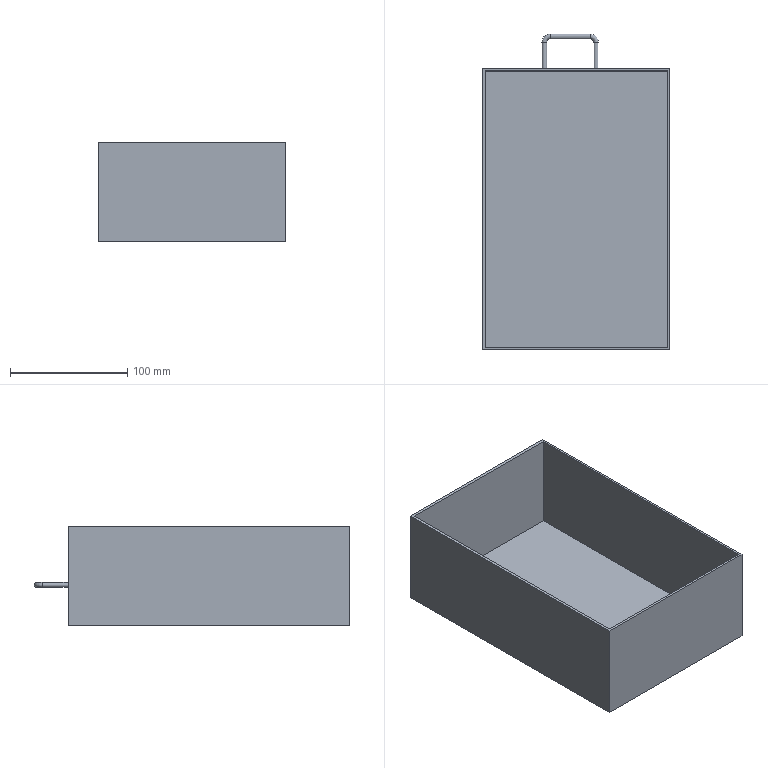Part | NX | features solid 2 | 1 solid | 16 faces | box 160 x 269 x 85 mm | volume 244007 mm3 | plane 11 | cylinder 3 | torus 2 | commonest cylinder face diameters 4 x3
STEP:
#1=CARTESIAN_POINT('',(553.,305.,-243.));
#2=VERTEX_POINT('',#1);
#3=CARTESIAN_POINT('',(553.,305.,-245.));
#4=DIRECTION('',(0.,1.,0.));
#5=DIRECTION('',(0.,0.,1.));
#6=AXIS2_PLACEMENT_3D('',#3,#4,#5);
#7=CIRCLE('',#6,2.);
#8=EDGE_CURVE('',#2,#2,#7,.F.);
#9=ORIENTED_EDGE('',*,*,#8,.T.);
#10=EDGE_LOOP('',(#9));
#11=FACE_BOUND('',#10,.T.);
#12=CARTESIAN_POINT('',(500.,305.,-195.));
#13=VERTEX_POINT('',#12);
#14=CARTESIAN_POINT('',(660.,305.,-195.));
#15=VERTEX_POINT('',#14);
#16=CARTESIAN_POINT('',(210.,305.,-195.));
#17=DIRECTION('',(1.,0.,0.));
#18=VECTOR('',#17,1000.);
#19=LINE('',#16,#18);
#20=EDGE_CURVE('',#13,#15,#19,.T.);
#21=ORIENTED_EDGE('',*,*,#20,.T.);
#22=CARTESIAN_POINT('',(660.,305.,-280.));
#23=VERTEX_POINT('',#22);
#24=CARTESIAN_POINT('',(660.,305.,-160.));
#25=DIRECTION('',(0.,0.,1.));
#26=VECTOR('',#25,1000.);
#27=LINE('',#24,#26);
#28=EDGE_CURVE('',#15,#23,#27,.F.);
#29=ORIENTED_EDGE('',*,*,#28,.T.);
#30=CARTESIAN_POINT('',(500.,305.,-280.));
#31=VERTEX_POINT('',#30);
#32=CARTESIAN_POINT('',(702.5,305.,-280.));
#33=DIRECTION('',(1.,0.,0.));
#34=VECTOR('',#33,1000.);
#35=LINE('',#32,#34);
#36=EDGE_CURVE('',#31,#23,#35,.T.);
#37=ORIENTED_EDGE('',*,*,#36,.F.);
#38=CARTESIAN_POINT('',(500.,305.,-160.));
#39=DIRECTION('',(0.,0.,-1.));
#40=VECTOR('',#39,1000.);
#41=LINE('',#38,#40);
#42=EDGE_CURVE('',#13,#31,#41,.T.);
#43=ORIENTED_EDGE('',*,*,#42,.F.);
#44=EDGE_LOOP('',(#21,#29,#37,#43));
#45=FACE_BOUND('',#44,.T.);
#46=CARTESIAN_POINT('',(597.,305.,-247.));
#47=VERTEX_POINT('',#46);
#48=CARTESIAN_POINT('',(597.,305.,-245.));
#49=DIRECTION('',(0.,-1.,0.));
#50=DIRECTION('',(0.,0.,-1.));
#51=AXIS2_PLACEMENT_3D('',#48,#49,#50);
#52=CIRCLE('',#51,2.);
#53=EDGE_CURVE('',#47,#47,#52,.F.);
#54=ORIENTED_EDGE('',*,*,#53,.F.);
#55=EDGE_LOOP('',(#54));
#56=FACE_BOUND('',#55,.T.);
#57=CARTESIAN_POINT('',(485.,305.,-160.));
#58=DIRECTION('',(0.,-1.,0.));
#59=DIRECTION('',(0.,0.,1.));
#60=AXIS2_PLACEMENT_3D('',#57,#58,#59);
#61=PLANE('',#60);
#62=ADVANCED_FACE('',(#11,#45,#56),#61,.F.);
#63=CARTESIAN_POINT('',(660.,65.,-195.));
#64=VERTEX_POINT('',#63);
#65=CARTESIAN_POINT('',(660.,0.,-195.));
#66=DIRECTION('',(0.,1.,0.));
#67=VECTOR('',#66,1000.);
#68=LINE('',#65,#67);
#69=EDGE_CURVE('',#15,#64,#68,.F.);
#70=ORIENTED_EDGE('',*,*,#69,.T.);
#71=CARTESIAN_POINT('',(660.,65.,-280.));
#72=VERTEX_POINT('',#71);
#73=CARTESIAN_POINT('',(660.,65.,-140.));
#74=DIRECTION('',(0.,0.,-1.));
#75=VECTOR('',#74,1000.);
#76=LINE('',#73,#75);
#77=EDGE_CURVE('',#64,#72,#76,.T.);
#78=ORIENTED_EDGE('',*,*,#77,.T.);
#79=CARTESIAN_POINT('',(660.,0.,-280.));
#80=DIRECTION('',(0.,1.,0.));
#81=VECTOR('',#80,1000.);
#82=LINE('',#79,#81);
#83=EDGE_CURVE('',#23,#72,#82,.F.);
#84=ORIENTED_EDGE('',*,*,#83,.F.);
#85=ORIENTED_EDGE('',*,*,#28,.F.);
#86=EDGE_LOOP('',(#70,#78,#84,#85));
#87=FACE_BOUND('',#86,.T.);
#88=CARTESIAN_POINT('',(660.,0.,-57.002));
#89=DIRECTION('',(-1.,0.,0.));
#90=DIRECTION('',(0.,0.,1.));
#91=AXIS2_PLACEMENT_3D('',#88,#89,#90);
#92=PLANE('',#91);
#93=ADVANCED_FACE('',(#87),#92,.F.);
#94=CARTESIAN_POINT('',(500.,65.,-195.));
#95=VERTEX_POINT('',#94);
#96=CARTESIAN_POINT('',(500.,0.,-195.));
#97=DIRECTION('',(0.,1.,0.));
#98=VECTOR('',#97,1000.);
#99=LINE('',#96,#98);
#100=EDGE_CURVE('',#95,#13,#99,.T.);
#101=ORIENTED_EDGE('',*,*,#100,.T.);
#102=ORIENTED_EDGE('',*,*,#42,.T.);
#103=CARTESIAN_POINT('',(500.,65.,-280.));
#104=VERTEX_POINT('',#103);
#105=CARTESIAN_POINT('',(500.,-47.5,-280.));
#106=DIRECTION('',(0.,1.,0.));
#107=VECTOR('',#106,1000.);
#108=LINE('',#105,#107);
#109=EDGE_CURVE('',#104,#31,#108,.T.);
#110=ORIENTED_EDGE('',*,*,#109,.F.);
#111=CARTESIAN_POINT('',(500.,65.,-160.));
#112=DIRECTION('',(0.,0.,1.));
#113=VECTOR('',#112,1000.);
#114=LINE('',#111,#113);
#115=EDGE_CURVE('',#95,#104,#114,.F.);
#116=ORIENTED_EDGE('',*,*,#115,.F.);
#117=EDGE_LOOP('',(#101,#102,#110,#116));
#118=FACE_BOUND('',#117,.T.);
#119=CARTESIAN_POINT('',(500.,302.5,-160.));
#120=DIRECTION('',(1.,0.,0.));
#121=DIRECTION('',(0.,0.,-1.));
#122=AXIS2_PLACEMENT_3D('',#119,#120,#121);
#123=PLANE('',#122);
#124=ADVANCED_FACE('',(#118),#123,.F.);
#125=CARTESIAN_POINT('',(-430.,65.,-195.));
#126=DIRECTION('',(1.,0.,0.));
#127=VECTOR('',#126,1000.);
#128=LINE('',#125,#127);
#129=EDGE_CURVE('',#64,#95,#128,.F.);
#130=ORIENTED_EDGE('',*,*,#129,.T.);
#131=ORIENTED_EDGE('',*,*,#115,.T.);
#132=CARTESIAN_POINT('',(-430.,65.,-280.));
#133=DIRECTION('',(1.,0.,0.));
#134=VECTOR('',#133,1000.);
#135=LINE('',#132,#134);
#136=EDGE_CURVE('',#72,#104,#135,.F.);
#137=ORIENTED_EDGE('',*,*,#136,.F.);
#138=ORIENTED_EDGE('',*,*,#77,.F.);
#139=EDGE_LOOP('',(#130,#131,#137,#138));
#140=FACE_BOUND('',#139,.T.);
#141=CARTESIAN_POINT('',(-430.,65.,-140.));
#142=DIRECTION('',(0.,1.,0.));
#143=DIRECTION('',(1.,0.,0.));
#144=AXIS2_PLACEMENT_3D('',#141,#142,#143);
#145=PLANE('',#144);
#146=ADVANCED_FACE('',(#140),#145,.F.);
#147=ORIENTED_EDGE('',*,*,#136,.T.);
#148=ORIENTED_EDGE('',*,*,#109,.T.);
#149=ORIENTED_EDGE('',*,*,#36,.T.);
#150=ORIENTED_EDGE('',*,*,#83,.T.);
#151=EDGE_LOOP('',(#147,#148,#149,#150));
#152=FACE_BOUND('',#151,.T.);
#153=CARTESIAN_POINT('',(702.5,-47.5,-280.));
#154=DIRECTION('',(0.,0.,1.));
#155=DIRECTION('',(1.,0.,0.));
#156=AXIS2_PLACEMENT_3D('',#153,#154,#155);
#157=PLANE('',#156);
#158=ADVANCED_FACE('',(#152),#157,.F.);
#159=CARTESIAN_POINT('',(658.,302.5,-195.));
#160=VERTEX_POINT('',#159);
#161=CARTESIAN_POINT('',(502.5,302.5,-195.));
#162=VERTEX_POINT('',#161);
#163=CARTESIAN_POINT('',(210.,302.5,-195.));
#164=DIRECTION('',(-1.,0.,0.));
#165=VECTOR('',#164,1000.);
#166=LINE('',#163,#165);
#167=EDGE_CURVE('',#160,#162,#166,.T.);
#168=ORIENTED_EDGE('',*,*,#167,.F.);
#169=CARTESIAN_POINT('',(658.,67.,-195.));
#170=VERTEX_POINT('',#169);
#171=CARTESIAN_POINT('',(658.,0.,-195.));
#172=DIRECTION('',(0.,1.,0.));
#173=VECTOR('',#172,1000.);
#174=LINE('',#171,#173);
#175=EDGE_CURVE('',#170,#160,#174,.T.);
#176=ORIENTED_EDGE('',*,*,#175,.F.);
#177=CARTESIAN_POINT('',(502.5,67.,-195.));
#178=VERTEX_POINT('',#177);
#179=CARTESIAN_POINT('',(210.,67.,-195.));
#180=DIRECTION('',(1.,0.,0.));
#181=VECTOR('',#180,1000.);
#182=LINE('',#179,#181);
#183=EDGE_CURVE('',#178,#170,#182,.T.);
#184=ORIENTED_EDGE('',*,*,#183,.F.);
#185=CARTESIAN_POINT('',(502.5,0.,-195.));
#186=DIRECTION('',(0.,-1.,0.));
#187=VECTOR('',#186,1000.);
#188=LINE('',#185,#187);
#189=EDGE_CURVE('',#162,#178,#188,.T.);
#190=ORIENTED_EDGE('',*,*,#189,.F.);
#191=EDGE_LOOP('',(#168,#176,#184,#190));
#192=FACE_BOUND('',#191,.T.);
#193=ORIENTED_EDGE('',*,*,#100,.F.);
#194=ORIENTED_EDGE('',*,*,#129,.F.);
#195=ORIENTED_EDGE('',*,*,#69,.F.);
#196=ORIENTED_EDGE('',*,*,#20,.F.);
#197=EDGE_LOOP('',(#193,#194,#195,#196));
#198=FACE_BOUND('',#197,.T.);
#199=CARTESIAN_POINT('',(210.,0.,-195.));
#200=DIRECTION('',(0.,0.,1.));
#201=DIRECTION('',(1.,0.,0.));
#202=AXIS2_PLACEMENT_3D('',#199,#200,#201);
#203=PLANE('',#202);
#204=ADVANCED_FACE('',(#192,#198),#203,.T.);
#205=CARTESIAN_POINT('',(658.,302.5,-277.5));
#206=VERTEX_POINT('',#205);
#207=CARTESIAN_POINT('',(658.,67.,-277.5));
#208=VERTEX_POINT('',#207);
#209=CARTESIAN_POINT('',(658.,-47.5,-277.5));
#210=DIRECTION('',(0.,-1.,0.));
#211=VECTOR('',#210,1000.);
#212=LINE('',#209,#211);
#213=EDGE_CURVE('',#206,#208,#212,.T.);
#214=ORIENTED_EDGE('',*,*,#213,.F.);
#215=CARTESIAN_POINT('',(502.5,302.5,-277.5));
#216=VERTEX_POINT('',#215);
#217=CARTESIAN_POINT('',(705.,302.5,-277.5));
#218=DIRECTION('',(1.,0.,0.));
#219=VECTOR('',#218,1000.);
#220=LINE('',#217,#219);
#221=EDGE_CURVE('',#216,#206,#220,.T.);
#222=ORIENTED_EDGE('',*,*,#221,.F.);
#223=CARTESIAN_POINT('',(502.5,67.,-277.5));
#224=VERTEX_POINT('',#223);
#225=CARTESIAN_POINT('',(502.5,302.5,-277.5));
#226=DIRECTION('',(0.,1.,0.));
#227=VECTOR('',#226,1000.);
#228=LINE('',#225,#227);
#229=EDGE_CURVE('',#224,#216,#228,.T.);
#230=ORIENTED_EDGE('',*,*,#229,.F.);
#231=CARTESIAN_POINT('',(485.,67.,-277.5));
#232=DIRECTION('',(-1.,0.,0.));
#233=VECTOR('',#232,1000.);
#234=LINE('',#231,#233);
#235=EDGE_CURVE('',#208,#224,#234,.T.);
#236=ORIENTED_EDGE('',*,*,#235,.F.);
#237=EDGE_LOOP('',(#214,#222,#230,#236));
#238=FACE_BOUND('',#237,.T.);
#239=CARTESIAN_POINT('',(702.5,-47.5,-277.5));
#240=DIRECTION('',(0.,0.,1.));
#241=DIRECTION('',(1.,0.,0.));
#242=AXIS2_PLACEMENT_3D('',#239,#240,#241);
#243=PLANE('',#242);
#244=ADVANCED_FACE('',(#238),#243,.T.);
#245=ORIENTED_EDGE('',*,*,#175,.T.);
#246=CARTESIAN_POINT('',(658.,302.5,-160.));
#247=DIRECTION('',(0.,0.,-1.));
#248=VECTOR('',#247,1000.);
#249=LINE('',#246,#248);
#250=EDGE_CURVE('',#160,#206,#249,.T.);
#251=ORIENTED_EDGE('',*,*,#250,.T.);
#252=ORIENTED_EDGE('',*,*,#213,.T.);
#253=CARTESIAN_POINT('',(658.,67.,-160.));
#254=DIRECTION('',(0.,0.,-1.));
#255=VECTOR('',#254,1000.);
#256=LINE('',#253,#255);
#257=EDGE_CURVE('',#170,#208,#256,.T.);
#258=ORIENTED_EDGE('',*,*,#257,.F.);
#259=EDGE_LOOP('',(#245,#251,#252,#258));
#260=FACE_BOUND('',#259,.T.);
#261=CARTESIAN_POINT('',(658.,-47.5,-160.));
#262=DIRECTION('',(1.,0.,0.));
#263=DIRECTION('',(0.,0.,-1.));
#264=AXIS2_PLACEMENT_3D('',#261,#262,#263);
#265=PLANE('',#264);
#266=ADVANCED_FACE('',(#260),#265,.F.);
#267=ORIENTED_EDGE('',*,*,#189,.T.);
#268=CARTESIAN_POINT('',(502.5,67.,-160.));
#269=DIRECTION('',(0.,0.,-1.));
#270=VECTOR('',#269,1000.);
#271=LINE('',#268,#270);
#272=EDGE_CURVE('',#178,#224,#271,.T.);
#273=ORIENTED_EDGE('',*,*,#272,.T.);
#274=ORIENTED_EDGE('',*,*,#229,.T.);
#275=CARTESIAN_POINT('',(502.5,302.5,-160.));
#276=DIRECTION('',(0.,0.,-1.));
#277=VECTOR('',#276,1000.);
#278=LINE('',#275,#277);
#279=EDGE_CURVE('',#162,#216,#278,.T.);
#280=ORIENTED_EDGE('',*,*,#279,.F.);
#281=EDGE_LOOP('',(#267,#273,#274,#280));
#282=FACE_BOUND('',#281,.T.);
#283=CARTESIAN_POINT('',(502.5,302.5,-160.));
#284=DIRECTION('',(-1.,0.,0.));
#285=DIRECTION('',(0.,0.,1.));
#286=AXIS2_PLACEMENT_3D('',#283,#284,#285);
#287=PLANE('',#286);
#288=ADVANCED_FACE('',(#282),#287,.F.);
#289=ORIENTED_EDGE('',*,*,#183,.T.);
#290=ORIENTED_EDGE('',*,*,#257,.T.);
#291=ORIENTED_EDGE('',*,*,#235,.T.);
#292=ORIENTED_EDGE('',*,*,#272,.F.);
#293=EDGE_LOOP('',(#289,#290,#291,#292));
#294=FACE_BOUND('',#293,.T.);
#295=CARTESIAN_POINT('',(485.,67.,-160.));
#296=DIRECTION('',(0.,-1.,0.));
#297=DIRECTION('',(0.,0.,1.));
#298=AXIS2_PLACEMENT_3D('',#295,#296,#297);
#299=PLANE('',#298);
#300=ADVANCED_FACE('',(#294),#299,.F.);
#301=ORIENTED_EDGE('',*,*,#167,.T.);
#302=ORIENTED_EDGE('',*,*,#279,.T.);
#303=ORIENTED_EDGE('',*,*,#221,.T.);
#304=ORIENTED_EDGE('',*,*,#250,.F.);
#305=EDGE_LOOP('',(#301,#302,#303,#304));
#306=FACE_BOUND('',#305,.T.);
#307=CARTESIAN_POINT('',(705.,302.5,-160.));
#308=DIRECTION('',(0.,1.,0.));
#309=DIRECTION('',(0.,0.,-1.));
#310=AXIS2_PLACEMENT_3D('',#307,#308,#309);
#311=PLANE('',#310);
#312=ADVANCED_FACE('',(#306),#311,.F.);
#313=CARTESIAN_POINT('',(558.,332.,-247.));
#314=VERTEX_POINT('',#313);
#315=CARTESIAN_POINT('',(558.,332.,-245.));
#316=DIRECTION('',(1.,0.,0.));
#317=DIRECTION('',(0.,0.,-1.));
#318=AXIS2_PLACEMENT_3D('',#315,#316,#317);
#319=CIRCLE('',#318,2.);
#320=EDGE_CURVE('',#314,#314,#319,.T.);
#321=ORIENTED_EDGE('',*,*,#320,.F.);
#322=EDGE_LOOP('',(#321));
#323=FACE_BOUND('',#322,.T.);
#324=CARTESIAN_POINT('',(553.,327.,-247.));
#325=VERTEX_POINT('',#324);
#326=CARTESIAN_POINT('',(553.,327.,-245.));
#327=DIRECTION('',(0.,1.,0.));
#328=DIRECTION('',(0.,0.,-1.));
#329=AXIS2_PLACEMENT_3D('',#326,#327,#328);
#330=CIRCLE('',#329,2.);
#331=EDGE_CURVE('',#325,#325,#330,.T.);
#332=ORIENTED_EDGE('',*,*,#331,.T.);
#333=EDGE_LOOP('',(#332));
#334=FACE_BOUND('',#333,.T.);
#335=CARTESIAN_POINT('',(558.,327.,-245.));
#336=DIRECTION('',(0.,0.,-1.));
#337=DIRECTION('',(-1.,0.,0.));
#338=AXIS2_PLACEMENT_3D('',#335,#336,#337);
#339=TOROIDAL_SURFACE('',#338,5.,2.);
#340=ADVANCED_FACE('',(#323,#334),#339,.T.);
#341=ORIENTED_EDGE('',*,*,#331,.F.);
#342=EDGE_LOOP('',(#341));
#343=FACE_BOUND('',#342,.T.);
#344=ORIENTED_EDGE('',*,*,#8,.F.);
#345=EDGE_LOOP('',(#344));
#346=FACE_BOUND('',#345,.T.);
#347=CARTESIAN_POINT('',(553.,327.,-245.));
#348=DIRECTION('',(0.,-1.,0.));
#349=DIRECTION('',(0.,0.,1.));
#350=AXIS2_PLACEMENT_3D('',#347,#348,#349);
#351=CYLINDRICAL_SURFACE('',#350,2.);
#352=ADVANCED_FACE('',(#343,#346),#351,.T.);
#353=CARTESIAN_POINT('',(592.,332.,-247.));
#354=VERTEX_POINT('',#353);
#355=CARTESIAN_POINT('',(592.,332.,-245.));
#356=DIRECTION('',(1.,0.,0.));
#357=DIRECTION('',(0.,0.,-1.));
#358=AXIS2_PLACEMENT_3D('',#355,#356,#357);
#359=CIRCLE('',#358,2.);
#360=EDGE_CURVE('',#354,#354,#359,.T.);
#361=ORIENTED_EDGE('',*,*,#360,.F.);
#362=EDGE_LOOP('',(#361));
#363=FACE_BOUND('',#362,.T.);
#364=ORIENTED_EDGE('',*,*,#320,.T.);
#365=EDGE_LOOP('',(#364));
#366=FACE_BOUND('',#365,.T.);
#367=CARTESIAN_POINT('',(592.,332.,-245.));
#368=DIRECTION('',(-1.,0.,0.));
#369=DIRECTION('',(0.,0.,1.));
#370=AXIS2_PLACEMENT_3D('',#367,#368,#369);
#371=CYLINDRICAL_SURFACE('',#370,2.);
#372=ADVANCED_FACE('',(#363,#366),#371,.T.);
#373=CARTESIAN_POINT('',(597.,327.,-247.));
#374=VERTEX_POINT('',#373);
#375=CARTESIAN_POINT('',(597.,327.,-245.));
#376=DIRECTION('',(0.,-1.,0.));
#377=DIRECTION('',(0.,0.,-1.));
#378=AXIS2_PLACEMENT_3D('',#375,#376,#377);
#379=CIRCLE('',#378,2.);
#380=EDGE_CURVE('',#374,#374,#379,.T.);
#381=ORIENTED_EDGE('',*,*,#380,.F.);
#382=EDGE_LOOP('',(#381));
#383=FACE_BOUND('',#382,.T.);
#384=ORIENTED_EDGE('',*,*,#360,.T.);
#385=EDGE_LOOP('',(#384));
#386=FACE_BOUND('',#385,.T.);
#387=CARTESIAN_POINT('',(592.,327.,-245.));
#388=DIRECTION('',(0.,0.,-1.));
#389=DIRECTION('',(-1.,0.,0.));
#390=AXIS2_PLACEMENT_3D('',#387,#388,#389);
#391=TOROIDAL_SURFACE('',#390,5.,2.);
#392=ADVANCED_FACE('',(#383,#386),#391,.T.);
#393=ORIENTED_EDGE('',*,*,#380,.T.);
#394=EDGE_LOOP('',(#393));
#395=FACE_BOUND('',#394,.T.);
#396=ORIENTED_EDGE('',*,*,#53,.T.);
#397=EDGE_LOOP('',(#396));
#398=FACE_BOUND('',#397,.T.);
#399=CARTESIAN_POINT('',(597.,327.,-245.));
#400=DIRECTION('',(0.,-1.,0.));
#401=DIRECTION('',(0.,0.,1.));
#402=AXIS2_PLACEMENT_3D('',#399,#400,#401);
#403=CYLINDRICAL_SURFACE('',#402,2.);
#404=ADVANCED_FACE('',(#395,#398),#403,.T.);
#405=CLOSED_SHELL('',(#62,#93,#124,#146,#158,#204,#244,#266,#288,#300,#312,#340,#352,#372,#392,#404));
#406=MANIFOLD_SOLID_BREP('',#405);
#407=(LENGTH_UNIT()NAMED_UNIT(*)SI_UNIT(.MILLI.,.METRE.));
#408=UNCERTAINTY_MEASURE_WITH_UNIT(LENGTH_MEASURE(0.00001),#407,'','');
#409=(NAMED_UNIT(*)PLANE_ANGLE_UNIT()SI_UNIT($,.RADIAN.));
#410=(NAMED_UNIT(*)SI_UNIT($,.STERADIAN.)SOLID_ANGLE_UNIT());
#411=(GEOMETRIC_REPRESENTATION_CONTEXT(3)GLOBAL_UNCERTAINTY_ASSIGNED_CONTEXT((#408))GLOBAL_UNIT_ASSIGNED_CONTEXT((#407,#409,#410))REPRESENTATION_CONTEXT('',''));
#412=ADVANCED_BREP_SHAPE_REPRESENTATION('',(#406),#411);